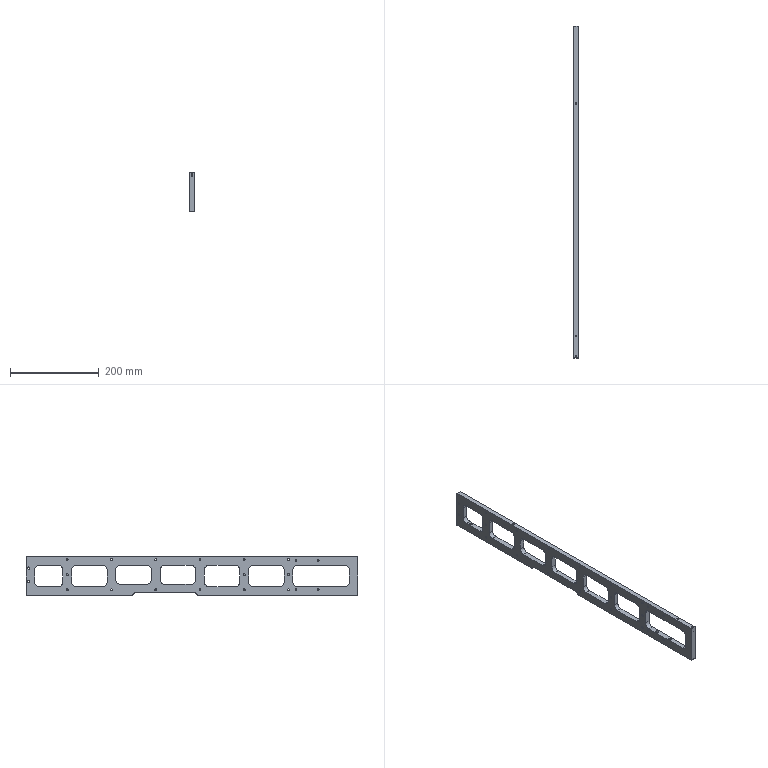CAM job | NX | 3+2 milling, drilling | part box 11 x 750 x 88 mm | stock box 15 x 755 x 93 mm
Tools:
number,name,description,diameter,corner_radius,flute_length,length,flutes
3,D3,平底铣刀-粗,3.0,0.0,20.0,75.0,2
9,D10,平底铣刀-粗,10.0,0.0,35.0,75.0,2
19,D3-J,平底铣刀-精,3.0,0.0,50.0,75.0,2
7,D6-J,平底铣刀-精,6.0,0.0,25.0,75.0,2
10,D10-J,平底铣刀-精,10.0,0.0,35.0,75.0,2
1,D80R0.8飞刀,圆鼻刀-粗,80.0,0.8,50.0,75.0,2
1,D80R0.8飞刀-J,圆鼻刀-精,80.0,0.8,50.0,75.0,2
2,D6倒角刀,倒角刀,6.0,0.0,3.0,25.0,2
22,M5X0.8,丝锥,4.2,0.0,35.0,50.0,2
18,M6X1.0,丝锥,5.0,0.0,35.0,50.0,2
15,ZT5,钻头,5.0,0.0,35.0,50.0,2
14,钻头4.2,Twist Drill 4.2 mm,4.2,0.0,41.0,41.738,2
17,ZT4.9,Drilling Tool,4.9,0.0,35.0,50.0,2
Operations:
program,operation,operation_type,tool,method,geometry_group,spindle_rpm,surface_speed,feed_per_tooth,feed_cut,feed_plunge,cut_length_mm,path_length_mm,cut_time_min,machine_time_min
B,底壁铣飞面开粗_COPY,VolumeBased25DMillingOperation,D80R0.8飞刀,分层开粗-切深K-步距G,W-B,2800.0,703.696,0.5357,3000.0,100.0,12061.735,12341.419,4.021,4.048
B,底壁铣飞面精光_COPY,VolumeBased25DMillingOperation,D80R0.8飞刀-J,侧刃精光-切深K-步距G,W-B,4000.0,1005.28,0.125,1000.0,100.0,1722.494,1758.494,1.722,1.726
B,打点-深0.8_2,Operation,D6倒角刀,NONE,W-B,8000.0,150.796,0.0312,500.0,90.0,5.4,552.806,0.0108,0.0655
B,通孔-精孔6.0预钻,Operation,ZT4.9,NONE,W-B,2500.0,38.484,0.05,250.0,90.0,24.0,590.006,0.096,0.1526
B,铣孔开粗D4_1,CylinderMilling,D3,NONE,W-B,8000.0,75.398,0.0312,500.0,100.0,463.149,1102.05,0.9263,0.9902
B,钻倒角_1,Operation,D6倒角刀,METHOD,W-B,5000.0,94.248,0.015,150.0,0.0,91.2,1308.334,0.608,0.7297
B,铣倒角_4,PlanarMilling,D6倒角刀,METHOD,W-B,8000.0,150.796,0.0312,500.0,100.0,58.471,685.296,0.1169,0.1796
B,C0.3封闭铣廓倒角6X45L_COPY,PlanarMilling,D6倒角刀,爬面_倒角-切深0-步距G,W-B,7000.0,131.0,0.1071,1500.0,100.0,3470.823,4685.002,2.314,2.435
B,铣孔精光D4-J_1,CylinderMilling,D3-J,精光步距切深关,W-B,8000.0,75.398,0.0125,200.0,100.0,170.583,809.483,0.8529,0.9168
A,顶面,FaceMilling,D80R0.8飞刀,侧刃精光-切深K-步距G,W-A,4000.0,1005.31,0.125,1000.0,100.0,2588,2624,2.588,2.592
A,外形粗_2,VolumeBased25DMillingOperation,D10,METHOD,W-A,8000.0,251.327,0.3125,5000.0,80.0,27379.949,27429.749,5.476,5.481
A,框开粗_1,VolumeBased25DMillingOperation,D10,METHOD,W-A,6000.0,188.0,0.25,4000.0,80.0,7220.41,7269.71,1.805,1.81
A,框开粗_2,VolumeBased25DMillingOperation,D10,METHOD,W-A,6000.0,188.0,0.25,4000.0,80.0,14893.243,15444.511,3.723,3.778
A,框开粗_3,VolumeBased25DMillingOperation,D10,METHOD,W-A,6000.0,188.0,0.25,4000.0,80.0,9448.831,9646.931,2.362,2.382
A,框开粗_4,VolumeBased25DMillingOperation,D10,METHOD,W-A,6000.0,188.0,0.25,4000.0,80.0,4148.417,4197.717,1.037,1.042
A,打点-深0.8,Operation,D6倒角刀,NONE,W-A,8000.0,150.796,0.0312,500.0,90.0,32.4,1280.627,0.0648,0.1896
A,通孔-M5螺纹底孔,Operation,钻头4.2,NONE,W-A,3000.0,39.584,0.0583,350.0,90.0,308.189,1711.132,0.8805,1.021
A,通孔-M6螺纹底孔,Operation,ZT5,NONE,W-A,2800.0,44.158,0.0625,350.0,90.0,39.004,149.025,0.1114,0.1224
A,框精_1,VolumeBased25DMillingOperation,D6-J,METHOD,W-A,6000.0,113.0,0.0833,1000.0,100.0,318.908,379.508,0.3189,0.325
A,框精_2,VolumeBased25DMillingOperation,D6-J,METHOD,W-A,6000.0,113.0,0.0833,1000.0,100.0,674.723,1261.523,0.6747,0.7334
A,框精_3,VolumeBased25DMillingOperation,D6-J,METHOD,W-A,6000.0,113.0,0.0833,1000.0,100.0,429.815,648.515,0.4298,0.4517
A,框精_4,VolumeBased25DMillingOperation,D6-J,METHOD,W-A,6000.0,113.0,0.0833,1000.0,100.0,190.908,251.508,0.1909,0.197
A,仅选体,SurfaceContour,D6倒角刀,METHOD,W-A,8000.0,150.796,0.1875,3000.0,100.0,3431.235,4661.169,1.144,1.267
A,铣倒角_1,PlanarMilling,D6倒角刀,METHOD,W-A,8000.0,150.796,0.0312,500.0,100.0,288.326,1977.074,0.5767,0.7455
A,铣倒角_2,PlanarMilling,D6倒角刀,METHOD,W-A,8000.0,150.796,0.0312,500.0,100.0,39.977,152.447,0.08,0.0912
A,通孔-攻牙M5,Operation,M5X0.8,METHOD,W-A,500.0,6.597,0.0008,0.8,90.0,248.0,1590.754,310.0,310.134
A,通孔-攻牙M6,Operation,M6X1.0,METHOD,W-A,500.0,7.854,0.001,1.0,90.0,31.0,133.017,31.0,31.01
A,外形半精_2,VolumeBased25DMillingOperation,D10-J,METHOD,W-A,8000.0,251.327,0.0625,1000.0,100.0,1715.524,1777.124,1.716,1.722